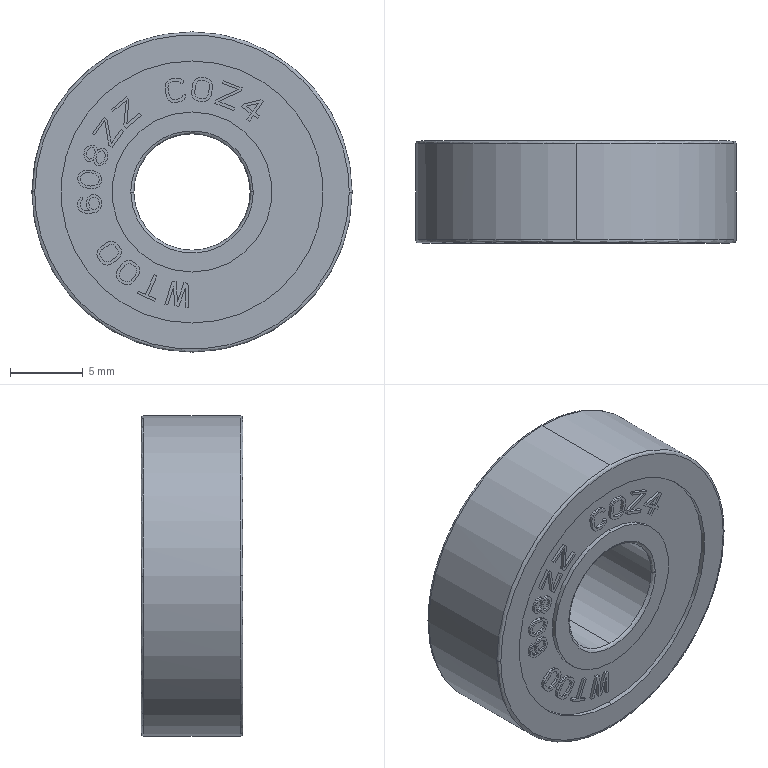Part | SolidWorks | features BaseBody 1 | 1 solid | 454 faces | box 22 x 7 x 22 mm | volume 2214 mm3 | plane 434 | cylinder 12 | spline 8 | commonest cylinder face diameters 11 x4 18 x4 8 x2 22 x2